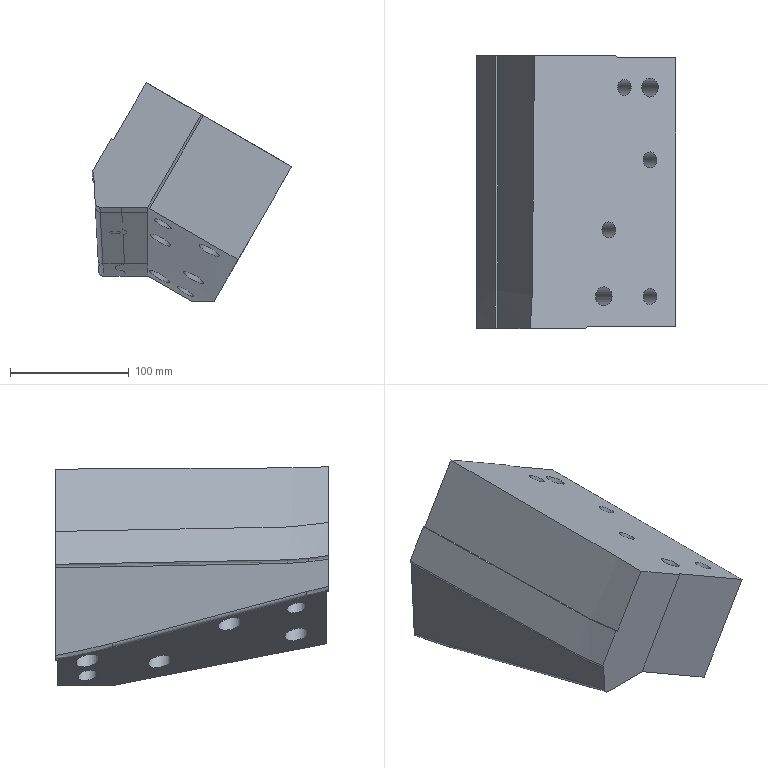Part | NX | features solid 2 | 1 solid | 41 faces | box 168.089 x 230 x 184.16 mm | volume 3580500 mm3 | spline 19 | plane 12 | cylinder 10 | commonest cylinder face diameters 13.5 x4 19.5 x4 16 x2